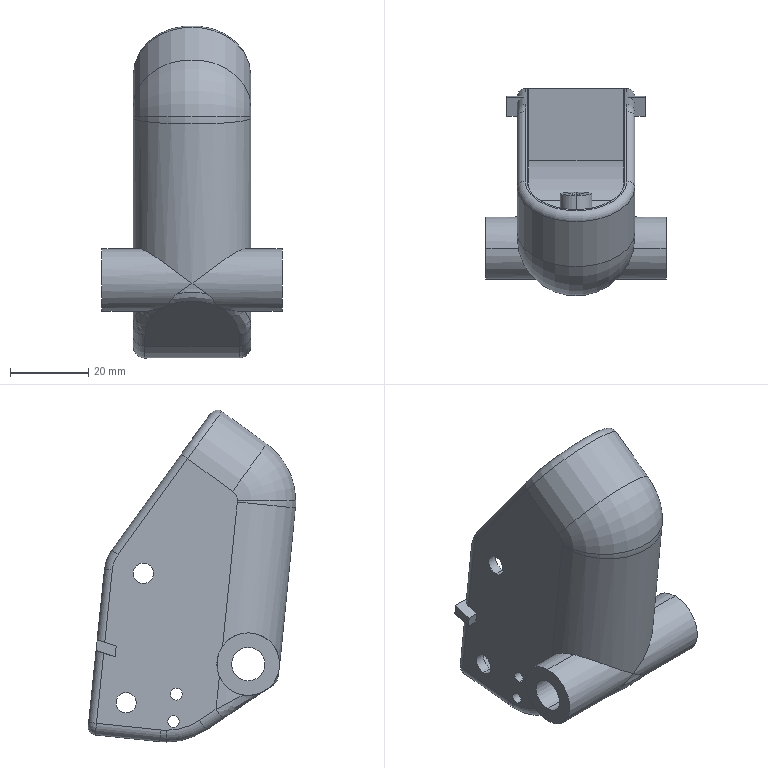Part | SolidWorks | features BaseBody 1 | 1 solid | 98 faces | box 46 x 53.095 x 84.854 mm | volume 26206 mm3 | cylinder 56 | plane 21 | torus 16 | spline 5 | commonest cylinder face diameters 4 x9 3 x8 5.2 x8 16 x6 30 x5 1 x4